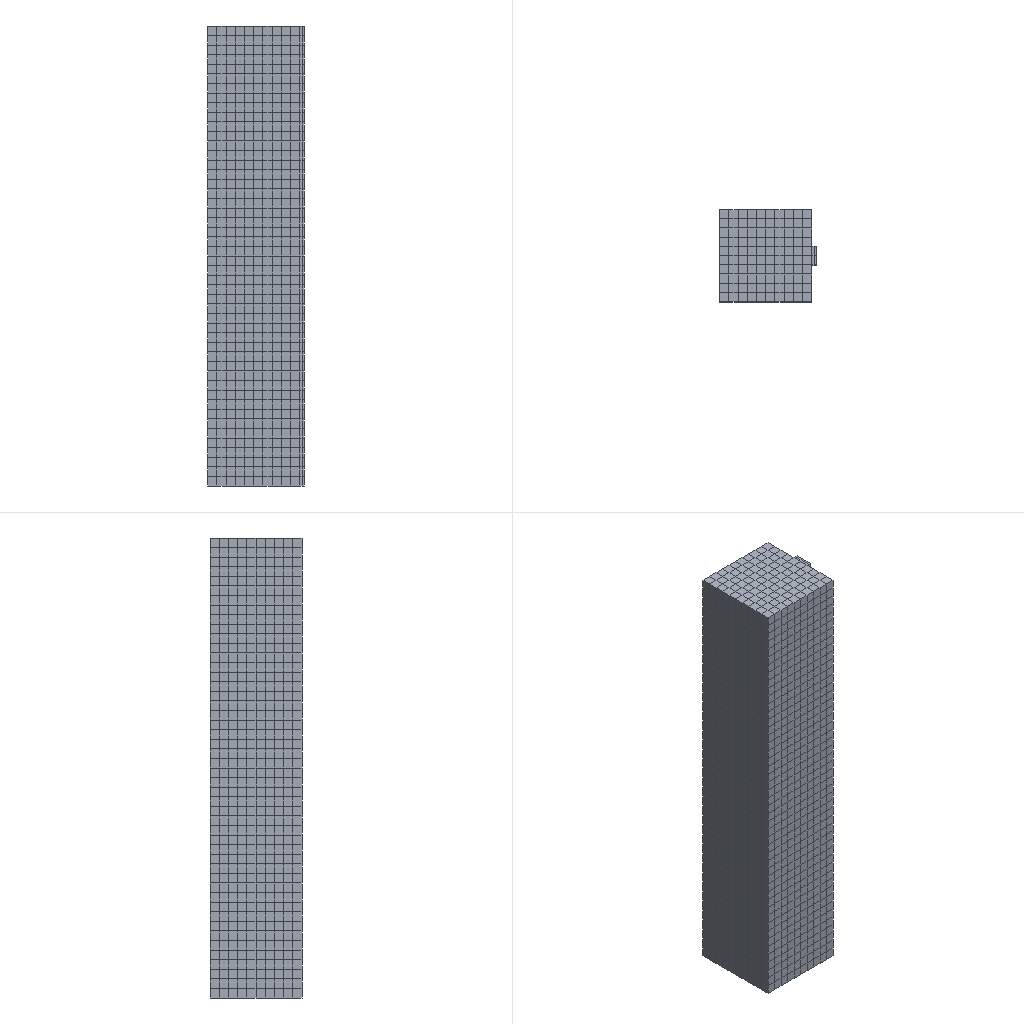Simulation study | abaqus
Set-up summary:
category,name,step,type,value,unit,region
solver,abaqus
solver,version,,,Abaqus/Explicit 2020
units,not stated in the deck,,not stated
analysis,deck,,transient,transient
load_step,Step-1,Step-1,transient
load_step,requested,,,1
mesh,nodes,,,8278
mesh,elements,,,6828
element_type,R3D4,,rigid,1440
element_type,T3D2,,truss,200
element_type,C3D8R,,solid,4992
element_type,COH3D8,,cohesive,196
load,load commands in deck,,count,1
bc,support commands in deck,,count,7
material,C30,,in results
material,EPOXY_2592,,in results
material,FIBER,,in results
material,CONCRETE COHESIVE,,in results
material,CONCRETE COHESIVE-COPY,,in results
check,setup vs results,,match,"per instance, exact: element labels, types and connectivity; labels of the nodes the elements use; coordinates of those nodes at SINGLE_PRECISION in 2 of 5 instance(s)"
Abaqus input file, long lists of numbers shortened:
*Heading
** Job name: Job-1 Model name: Model-1
** Generated by: Abaqus/CAE 2020
*Preprint, echo=NO, model=NO, history=NO, contact=NO
**
** PARTS
**
*Part, name=Part-1
*Node
      1,         105.,          60.,       -187.5
      2,         105.,          40.,       -187.5
** (6491 more lines like these left out)
*Element, type=C3D8R
 1,   8, 103, 820, 110,   1,  91, 815, 102
 2, 103,   5, 108, 820,  91,   2,  92, 815
** (4990 more lines like these left out)
*Element, type=COH3D8
4993,   71,  535, 1664,  574, 6227, 6226, 6225, 6224
4994,  535,  536, 1665, 1664, 6226, 6229, 6228, 6225
** (194 more lines like these left out)
*Nset, nset=Set-1
    1,    2,    3,    4,    5,    6,    7,    8,    9,   10,   11,   12,   13,   14,   15,   16
   17,   18,   19,   20,   21,   22,   23,   24,   25,   26,   27,   28,   29,   30,   31,   32
** (26 more lines like these left out)
*Elset, elset=Set-1, generate
   1,  192,    1
*Nset, nset=Set-5
   37,   38,   39,   40,   41,   42,   43,   44,   45,   46,   47,   48,   49,   50,   51,   52
   53,   54,   55,   56,   57,   58,   59,   60,   61,   62,   63,   64,   65,   66,   67,   68
** (377 more lines like these left out)
*Elset, elset=Set-5, generate
  193,  4992,     1
*Elset, elset=CohesiveSeam-1-Elements, generate
 4993,  5092,     1
*Nset, nset=CohesiveSeam-1-TopNodes
 6224, 6225, 6226, 6227, 6228, 6229, 6230, 6231, 6232, 6233, 6234, 6235, 6236, 6237, 6238, 6239
 6240, 6241, 6242, 6243, 6244, 6245, 6246, 6247, 6248, 6249, 6250, 6251, 6252, 6253, 6254, 6255
** (6 more lines like these left out)
*Nset, nset=CohesiveSeam-1-BottomNodes
   45,   46,   71,   72,   73,   74,  278,  535,  536,  537,  538,  539,  540,  551,  552,  553
  554,  555,  556,  557,  558,  559,  565,  566,  567,  568,  569,  570,  571,  572,  573,  574
** (6 more lines like these left out)
*Elset, elset=jiao-2-Elements, generate
 5093,  5188,     1
*Nset, nset=jiao-2-TopNodes
 6342, 6343, 6344, 6345, 6346, 6347, 6348, 6349, 6350, 6351, 6352, 6353, 6354, 6355, 6356, 6357
 6358, 6359, 6360, 6361, 6362, 6363, 6364, 6365, 6366, 6367, 6368, 6369, 6370, 6371, 6372, 6373
** (8 more lines like these left out)
*Nset, nset=jiao-2-BottomNodes
   37,   38,   39,   40,   41,   42,   43,   44,   45,   46,   47,   48,   49,   50,   51,   52
   53,   54,  249,  250,  251,  252,  253,  254,  255,  256,  257,  258,  259,  260,  261,  262
** (8 more lines like these left out)
*Elset, elset=__PickedSurf3_#9_S1, internal, generate
 4993,  5092,     1
*Surface, type=ELEMENT, name=_PickedSurf3_#9, internal
__PickedSurf3_#9_S1, S1
*Elset, elset=__PickedSurf15_#10_S1, internal, generate
 4993,  5092,     1
*Surface, type=ELEMENT, name=_PickedSurf15_#10, internal
__PickedSurf15_#10_S1, S1
*Elset, elset=__PickedSurf8_S1, internal, generate
 4993,  5092,     1
*Surface, type=ELEMENT, name=_PickedSurf8, internal
__PickedSurf8_S1, S1
*Elset, elset=__PickedSurf15_S1, internal, generate
 5093,  5188,     1
*Surface, type=ELEMENT, name=_PickedSurf15, internal
__PickedSurf15_S1, S1
*Elset, elset=_CohesiveSeam-1-TopSurf_S2, internal, generate
 4993,  5092,     1
*Surface, type=ELEMENT, name=CohesiveSeam-1-TopSurf
_CohesiveSeam-1-TopSurf_S2, S2
*Elset, elset=_CohesiveSeam-1-BottomSurf_S1, internal, generate
 4993,  5092,     1
*Surface, type=ELEMENT, name=CohesiveSeam-1-BottomSurf
_CohesiveSeam-1-BottomSurf_S1, S1
*Elset, elset=_jiao-2-TopSurf_S2, internal, generate
 5093,  5188,     1
*Surface, type=ELEMENT, name=jiao-2-TopSurf
_jiao-2-TopSurf_S2, S2
*Elset, elset=_jiao-2-BottomSurf_S1, internal, generate
 5093,  5188,     1
*Surface, type=ELEMENT, name=jiao-2-BottomSurf
_jiao-2-BottomSurf_S1, S1
** Section: adhesive
*Solid Section, elset=Set-1, material=Epoxy_2592
,
** Section: hnt
*Solid Section, elset=Set-5, material=C30
,
** Section: concrete cohesive
*Cohesive Section, elset=CohesiveSeam-1-Elements, controls=EC-1, material="concrete cohesive", response=TRACTION SEPARATION, thickness=SPECIFIED
0.1,
** Section: concrete cohesive-Copy
*Cohesive Section, elset=jiao-2-Elements, controls=EC-1, material="concrete cohesive-Copy", response=TRACTION SEPARATION, thickness=SPECIFIED
0.1,
*End Part
**
*Part, name=Part-2
*Node
      1,           0.,          25.,         150.
      2,           0.,          25.,           0.
** (525 more lines like these left out)
*Element, type=R3D4
  1,   1,   7, 122,  78
  2,   7,   8, 123, 122
** (478 more lines like these left out)
*Node
    528,           0., 1.53080845e-15,         150.
*Nset, nset=Part-2-RefPt_, internal
528,
*End Part
**
*Part, name=fiber
*Node
      1,        -250.,           0.,           0.
      2,       -247.5,           0.,           0.
** (199 more lines like these left out)
*Element, type=T3D2
  1,   1,   2
  2,   2,   3
** (198 more lines like these left out)
*Nset, nset=Set-2, generate
   1,  201,    1
*Elset, elset=Set-2, generate
   1,  200,    1
** Section: fiber
*Solid Section, elset=Set-2, material=fiber
1.,
*End Part
**
**
** ASSEMBLY
**
*Assembly, name=Assembly
**
*Instance, name=Part-2-1, part=Part-2
        -25.,         -25.,        187.5
        -25.,         -25.,        187.5,         -25., -24.,        187.5, 90.
*End Instance
**
*Instance, name=Part-2-1-lin-2-1, part=Part-2
        -25.,         -25.,       -187.5
        -25.,         -25.,       -187.5,         -25., -24.,       -187.5, 90.
*End Instance
**
*Instance, name=Part-2-1-lin-3-1, part=Part-2
        -25.,         125.,           0.
        -25.,         125.,           0., -24.293,         125., 0.7071,         180.
*End Instance
**
*Instance, name=fiber-1, part=fiber
       102.5,          50.,           0.
       102.5,          50.,           0.,        102.5, 51.,           0., 90.
*End Instance
**
*Instance, name=Part-1-1, part=Part-1
*End Instance
**
*Nset, nset=Set-7, instance=Part-2-1
 528,
*Nset, nset=Set-7, instance=Part-2-1-lin-2-1
 528,
*Nset, nset=Set-8, instance=Part-2-1-lin-3-1
 528,
*Nset, nset=b_Set-1, instance=Part-2-1, generate
   1,  527,    1
*Elset, elset=b_Set-1, instance=Part-2-1, generate
   1,  480,    1
*Nset, nset=b_Set-3, instance=Part-2-1-lin-3-1, generate
   1,  527,    1
*Elset, elset=b_Set-3, instance=Part-2-1-lin-3-1, generate
   1,  480,    1
*Nset, nset=b_Set-5, instance=Part-2-1-lin-2-1, generate
   1,  527,    1
*Elset, elset=b_Set-5, instance=Part-2-1-lin-2-1, generate
   1,  480,    1
*Nset, nset=m_Set-9, instance=fiber-1, generate
   1,  201,    1
*Elset, elset=m_Set-9, instance=fiber-1, generate
   1,  200,    1
*Nset, nset=m_Set-11, instance=fiber-1, generate
   1,  201,    1
*Elset, elset=m_Set-11, instance=fiber-1, generate
   1,  200,    1
*Nset, nset=s_Set-9, instance=Part-1-1
    1,    2,    3,    4,    5,    6,    7,    8,    9,   10,   11,   12,   13,   14,   15,   16
   17,   18,   19,   20,   21,   22,   23,   24,   25,   26,   27,   28,   29,   30,   31,   32
** (26 more lines like these left out)
*Elset, elset=s_Set-9, instance=Part-1-1, generate
   1,  192,    1
*Nset, nset=s_Set-11, instance=Part-1-1
    1,    2,    3,    4,    5,    6,    7,    8,    9,   10,   11,   12,   13,   14,   15,   16
   17,   18,   19,   20,   21,   22,   23,   24,   25,   26,   27,   28,   29,   30,   31,   32
** (26 more lines like these left out)
*Elset, elset=s_Set-11, instance=Part-1-1, generate
   1,  192,    1
*Nset, nset=_PickedSet21, internal, instance=Part-2-1
 528,
*Nset, nset=_PickedSet23, internal, instance=Part-2-1-lin-3-1
 528,
*Nset, nset=_PickedSet25, internal, instance=Part-2-1-lin-2-1
 528,
*Elset, elset=_CP-1-Part-2-1_SNEG, internal, instance=Part-2-1, generate
   1,  480,    1
*Surface, type=ELEMENT, name=CP-1-Part-2-1
_CP-1-Part-2-1_SNEG, SNEG
*Elset, elset=_CP-1-concrete-buer-1_S3, internal, instance=Part-1-1
  193,  194,  195,  196,  197,  198,  253,  254,  255,  256,  257,  258,  313,  314,  315,  316
  317,  318,  373,  374,  375,  376,  377,  378,  433,  434,  435,  436,  437,  438,  493,  494
** (21 more lines like these left out)
*Elset, elset=_CP-1-concrete-buer-1_S1, internal, instance=Part-1-1
 1333, 1334, 1335, 1336, 1337, 1338, 1339, 1340, 1341, 1342, 1343, 1344, 1345, 1346, 1347, 1348
 1349, 1350, 1351, 1352, 1353, 1354, 1355, 1356, 1357, 1358, 1359, 1360, 1361, 1362, 1363, 1364
** (6 more lines like these left out)
*Surface, type=ELEMENT, name=CP-1-concrete-buer-1
_CP-1-concrete-buer-1_S3, S3
_CP-1-concrete-buer-1_S1, S1
*Elset, elset=_CP-2-Part-2-1-lin-2-1_SNEG, internal, instance=Part-2-1-lin-2-1, generate
   1,  480,    1
*Surface, type=ELEMENT, name=CP-2-Part-2-1-lin-2-1
_CP-2-Part-2-1-lin-2-1_SNEG, SNEG
*Elset, elset=_CP-2-concrete-buer-1_S3, internal, instance=Part-1-1
  193,  194,  195,  196,  197,  198,  253,  254,  255,  256,  257,  258,  313,  314,  315,  316
  317,  318,  373,  374,  375,  376,  377,  378,  433,  434,  435,  436,  437,  438,  493,  494
** (21 more lines like these left out)
*Elset, elset=_CP-2-concrete-buer-1_S1, internal, instance=Part-1-1
 1333, 1334, 1335, 1336, 1337, 1338, 1339, 1340, 1341, 1342, 1343, 1344, 1345, 1346, 1347, 1348
 1349, 1350, 1351, 1352, 1353, 1354, 1355, 1356, 1357, 1358, 1359, 1360, 1361, 1362, 1363, 1364
** (6 more lines like these left out)
*Surface, type=ELEMENT, name=CP-2-concrete-buer-1
_CP-2-concrete-buer-1_S3, S3
_CP-2-concrete-buer-1_S1, S1
*Elset, elset=_CP-3-Part-2-1-lin-3-1_SNEG, internal, instance=Part-2-1-lin-3-1, generate
   1,  480,    1
*Surface, type=ELEMENT, name=CP-3-Part-2-1-lin-3-1
_CP-3-Part-2-1-lin-3-1_SNEG, SNEG
*Elset, elset=_CP-3-concrete-buer-1_S5, internal, instance=Part-1-1
  247,  248,  249,  250,  251,  252,  307,  308,  309,  310,  311,  312,  367,  368,  369,  370
  371,  372,  427,  428,  429,  430,  431,  432,  487,  488,  489,  490,  491,  492,  547,  548
** (21 more lines like these left out)
*Elset, elset=_CP-3-concrete-buer-1_S2, internal, instance=Part-1-1
  793,  794,  795,  796,  797,  798,  799,  800,  801,  802,  803,  804,  805,  806,  807,  808
  809,  810,  811,  812,  813,  814,  815,  816,  817,  818,  819,  820,  821,  822,  823,  824
** (6 more lines like these left out)
*Surface, type=ELEMENT, name=CP-3-concrete-buer-1
_CP-3-concrete-buer-1_S5, S5
_CP-3-concrete-buer-1_S2, S2
*Elset, elset=_CP-4-adhesive-2_S1, internal, instance=Part-1-1, generate
 5093,  5188,     1
*Surface, type=ELEMENT, name=CP-4-adhesive-2
_CP-4-adhesive-2_S1, S1
*Elset, elset=_CP-4-concrete-buer-1_S2, internal, instance=Part-1-1
  193,  194,  195,  196,  197,  198,  199,  200,  201,  202,  203,  204,  205,  206,  207,  208
  209,  210,  211,  212,  213,  214,  215,  216,  229,  230,  231,  232,  233,  234,  235,  236
** (16 more lines like these left out)
*Elset, elset=_CP-4-concrete-buer-1_S1, internal, instance=Part-1-1, generate
 5093,  5188,     1
*Elset, elset=_CP-4-concrete-buer-1_S6, internal, instance=Part-1-1
  793,  803,  813,  823,  833,  843,  853,  863,  873,  883,  893,  903,  913,  923,  933,  943
  953,  963,  973,  983,  993, 1003, 1013, 1023, 1153, 1163, 1173, 1183, 1193, 1203, 1213, 1223
** (4 more lines like these left out)
*Surface, type=ELEMENT, name=CP-4-concrete-buer-1
_CP-4-concrete-buer-1_S2, S2
_CP-4-concrete-buer-1_S1, S1
_CP-4-concrete-buer-1_S6, S6
*Elset, elset=_m_Surf-9_S2, internal, instance=Part-1-1
  193,  194,  195,  196,  197,  198,  199,  200,  201,  202,  203,  204,  205,  206,  207,  208
  209,  210,  211,  212,  213,  214,  215,  216,  229,  230,  231,  232,  233,  234,  235,  236
** (16 more lines like these left out)
*Elset, elset=_m_Surf-9_S1, internal, instance=Part-1-1, generate
 5093,  5188,     1
*Elset, elset=_m_Surf-9_S6, internal, instance=Part-1-1
  793,  803,  813,  823,  833,  843,  853,  863,  873,  883,  893,  903,  913,  923,  933,  943
  953,  963,  973,  983,  993, 1003, 1013, 1023, 1153, 1163, 1173, 1183, 1193, 1203, 1213, 1223
** (4 more lines like these left out)
*Surface, type=ELEMENT, name=m_Surf-9
_m_Surf-9_S2, S2
_m_Surf-9_S1, S1
_m_Surf-9_S6, S6
*Elset, elset=_s_Surf-9_S1, internal, instance=Part-1-1, generate
 5093,  5188,     1
*Surface, type=ELEMENT, name=s_Surf-9
_s_Surf-9_S1, S1
** Constraint: Constraint-1
*Rigid Body, ref node=_PickedSet21, elset=b_Set-1, position=CENTER OF MASS
** Constraint: Constraint-2
*Rigid Body, ref node=_PickedSet23, elset=b_Set-3, position=CENTER OF MASS
** Constraint: Constraint-3
*Rigid Body, ref node=_PickedSet25, elset=b_Set-5, position=CENTER OF MASS
** Constraint: Constraint-6
*Embedded Element, host elset=s_Set-11
m_Set-11
*End Assembly
**
** ELEMENT CONTROLS
**
*Section Controls, name=EC-1, ELEMENT DELETION=YES
1., 1., 1.
*Amplitude, name=Amp-1, definition=SMOOTH STEP
             0.,              0.,             0.1,              1.
**
** MATERIALS
**
*Material, name=C30
*Density
 2.5e-09,
*Elastic
31500., 0.2
*Concrete Damaged Plasticity
30.,   0.1,  1.16, 0.667, 0.005
*Concrete Compression Hardening
 29.725,          0.
 31.404, 0.0003292
 32.417, 0.0004674
  32.756, 0.0006281
 32.308, 0.0008151
 31.173,  0.001025
 29.63,  0.001248
 27.898,  0.001478
 26.122,  0.001709
 24.393,  0.001939
 22.76,  0.002165
 21.245,  0.002388
 19.857,  0.002606
 18.591,  0.00282
 14.594,  0.003642
 11.854,  0.004421
 10.804,  0.0048
*Concrete Tension Stiffening
  2.041,          0.
  2.269, 9.96907e-06
  2.434, 1.51574e-05
      2.5, 2.36667e-05
  2.262, 5.30086e-05
  1.933, 8.53686e-05
  1.654, 0.0001161
  1.436, 0.0001447
  1.266, 0.0001718
  1.132, 0.0001977
  1.025, 0.0002226
 0.9372,  0.000247
  0.8646, 0.0002708
 0.8034, 0.0002942
*Concrete Compression Damage
       0.,          0.
 0.1278, 0.0003292
 0.1645, 0.0004674
 0.2033, 0.0006281
 0.2455, 0.0008151
 0.2905,  0.001025
 0.3354,  0.001248
 0.3786,  0.001478
 0.4191,  0.001709
 0.4564,  0.001939
  0.4906,  0.002165
 0.5217,  0.002388
 0.55,  0.002606
 0.5756,  0.00282
  0.6567,  0.003642
 0.7136,  0.004421
 0.7358,  0.0048
 0.7863,  0.005909
 0.8107,  0.006633
 0.8302,  0.00735
 0.8461,  0.00806
 0.8593,  0.008767
 0.8705,  0.00947
 0.88,   0.01017
 0.8883,   0.01087
 0.8954,   0.01157
 0.9018,   0.01226
 0.9074,   0.01296
 0.9124,   0.01365
 0.9169,   0.01435
 0.9209,   0.01504
   0.9246,    0.01573
 0.928,   0.01643
 0.931,   0.01712
 0.9338,   0.01781
 0.9364,    0.0185
 0.9431,   0.02057
 0.9516,   0.02402
 0.9579,   0.02747
 0.9628,   0.03092
** (1 more lines like these left out)
*Concrete Tension Damage
        0.,          0.
 0.06003, 9.96907e-06
  0.08207, 1.51574e-05
  0.1175, 2.36667e-05
  0.2337, 5.30086e-05
  0.3442, 8.53686e-05
    0.4325, 0.0001161
  0.5015, 0.0001447
  0.556, 0.0001718
  0.5996, 0.0001977
  0.6353, 0.0002226
  0.6649,  0.000247
  0.6899, 0.0002708
  0.7112, 0.0002942
  0.7296, 0.0003174
  0.7456, 0.0003403
  0.7598, 0.000363
  0.7723, 0.0003855
  0.7835, 0.0004079
  0.7936,  0.0004303
  0.8027, 0.0004525
  0.811, 0.0004746
   0.8186, 0.0004967
  0.8255, 0.0005187
   0.8319, 0.0005407
  0.8378,   0.0005626
  0.8433, 0.0005845
  0.8483, 0.0006063
   0.8531, 0.0006281
  0.9063, 0.0008485
  0.9334,  0.001065
  0.9494,  0.001281
  0.9597,  0.001496
  0.9669,  0.00171
  0.9721,   0.001924
  0.976,  0.002139
*Material, name=Epoxy_2592
*Damage Initiation, criterion=DUCTILE
 0.05, -0.333,     0.
*Damage Evolution, type=DISPLACEMENT
 0.15,
*Density
 1.2e-09,
*Elastic
3400., 0.31
*Plastic, hardening=JOHNSON COOK
120., 654.18,  0.772,  0.304,     0.,     0.
*Material, name="concrete cohesive"
*Damage Initiation, criterion=MAXS
10.,10.,10.
*Damage Evolution, type=DISPLACEMENT
 0.01,
*Density
 1.2e-09,
*Elastic, type=TRACTION
1000.,1000.,1000.
*Material, name="concrete cohesive-Copy"
*Damage Initiation, criterion=MAXS
1.,1.,1.
*Damage Evolution, type=DISPLACEMENT
 0.01,
*Density
 1.2e-09,
*Elastic, type=TRACTION
1000.,1000.,1000.
*Material, name=fiber
*Density
 2.5e-09,
*Elastic
72000., 0.3
**
** INTERACTION PROPERTIES
**
*Surface Interaction, name=IntProp-1
*Friction
 0.2,
*Surface Behavior, pressure-overclosure=HARD
**
** BOUNDARY CONDITIONS
**
** Name: BC-1 Type: 对称/反对称/完全固定
*Boundary
Set-7, ENCASTRE
** ----------------------------------------------------------------
**
** STEP: Step-1
**
*Step, name=Step-1, nlgeom=YES
*Dynamic, Explicit
, 0.1
*Bulk Viscosity
0.06, 1.2
**
** BOUNDARY CONDITIONS
**
** Name: BC-2 Type: 位移/转角
*Boundary, amplitude=Amp-1
Set-8, 1, 1
Set-8, 2, 2, -2.
Set-8, 3, 3
Set-8, 4, 4
Set-8, 5, 5
Set-8, 6, 6
**
** INTERACTIONS
**
** Interaction: Int-4
*Contact, op=NEW
*Contact Inclusions, ALL EXTERIOR
*Contact Property Assignment
 ,  , IntProp-1
**
** OUTPUT REQUESTS
**
*Restart, write, number interval=1, time marks=NO
**
** FIELD OUTPUT: F-Output-1
**
*Output, field, number interval=50
*Node Output
A, RF, U, V
*Element Output, directions=YES
DAMAGEC, DAMAGET, DMICRT, E, EVF, LE, MISES, PE, PEEQ, PEEQVAVG, PEVAVG, S, SDEG, STATUS, SVAVG
*Contact Output
CSTRESS,
**
** HISTORY OUTPUT: H-Output-1
**
*Output, history, variable=PRESELECT
*End Step
Results summary:
result,step,Step-1,completed,increments=374976 time=0.1/0.1
result,analysis,,,transient
result,last_loadstep,,,1
result,primary field,,,U
result,reaction total,,FX,0.0,model units
result,reaction total,,FY,0.0,model units
result,reaction total,,FZ,0.0,model units